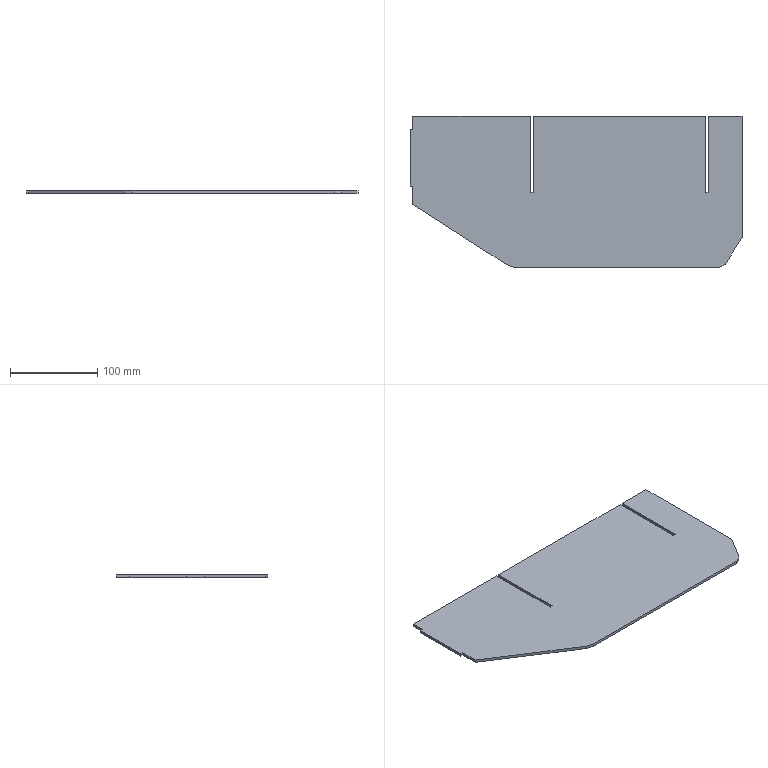Part | SolidWorks | features FlatPattern 1, SMBaseFlange 1, SheetMetal 1 | 1 solid | 22 faces | box 379.5 x 173.7 x 3.2 mm | volume 193629 mm3 | plane 22
STEP:
#1=CARTESIAN_POINT('',(-57.013,-111.363,0.));
#2=VERTEX_POINT('',#1);
#3=CARTESIAN_POINT('',(-47.809,-114.07,0.));
#4=VERTEX_POINT('',#3);
#5=CARTESIAN_POINT('',(-57.013,-111.363,0.));
#6=DIRECTION('',(0.9594,-0.2821,0.));
#7=VECTOR('',#6,1000.);
#8=LINE('',#5,#7);
#9=EDGE_CURVE('',#2,#4,#8,.T.);
#10=ORIENTED_EDGE('',*,*,#9,.T.);
#11=CARTESIAN_POINT('',(-47.809,-114.07,3.2));
#12=VERTEX_POINT('',#11);
#13=CARTESIAN_POINT('',(-47.809,-114.07,3.2));
#14=DIRECTION('',(0.,0.,-1.));
#15=VECTOR('',#14,1000.);
#16=LINE('',#13,#15);
#17=EDGE_CURVE('',#12,#4,#16,.T.);
#18=ORIENTED_EDGE('',*,*,#17,.F.);
#19=CARTESIAN_POINT('',(-57.013,-111.363,3.2));
#20=VERTEX_POINT('',#19);
#21=CARTESIAN_POINT('',(-57.013,-111.363,3.2));
#22=DIRECTION('',(0.9594,-0.2821,0.));
#23=VECTOR('',#22,1000.);
#24=LINE('',#21,#23);
#25=EDGE_CURVE('',#20,#12,#24,.T.);
#26=ORIENTED_EDGE('',*,*,#25,.F.);
#27=CARTESIAN_POINT('',(-57.013,-111.363,3.2));
#28=DIRECTION('',(0.,0.,-1.));
#29=VECTOR('',#28,1000.);
#30=LINE('',#27,#29);
#31=EDGE_CURVE('',#20,#2,#30,.T.);
#32=ORIENTED_EDGE('',*,*,#31,.T.);
#33=EDGE_LOOP('',(#10,#18,#26,#32));
#34=FACE_OUTER_BOUND('',#33,.T.);
#35=CARTESIAN_POINT('',(-57.013,-111.363,3.2));
#36=DIRECTION('',(0.2821,0.9594,0.));
#37=DIRECTION('',(-0.9594,0.2821,0.));
#38=AXIS2_PLACEMENT_3D('',#35,#36,#37);
#39=PLANE('',#38);
#40=ADVANCED_FACE('',(#34),#39,.F.);
#41=CARTESIAN_POINT('',(183.691,-114.07,0.));
#42=VERTEX_POINT('',#41);
#43=CARTESIAN_POINT('',(-47.809,-114.07,0.));
#44=DIRECTION('',(1.,0.,0.));
#45=VECTOR('',#44,1000.);
#46=LINE('',#43,#45);
#47=EDGE_CURVE('',#4,#42,#46,.T.);
#48=ORIENTED_EDGE('',*,*,#47,.T.);
#49=CARTESIAN_POINT('',(183.691,-114.07,3.2));
#50=VERTEX_POINT('',#49);
#51=CARTESIAN_POINT('',(183.691,-114.07,3.2));
#52=DIRECTION('',(0.,0.,-1.));
#53=VECTOR('',#52,1000.);
#54=LINE('',#51,#53);
#55=EDGE_CURVE('',#50,#42,#54,.T.);
#56=ORIENTED_EDGE('',*,*,#55,.F.);
#57=CARTESIAN_POINT('',(-47.809,-114.07,3.2));
#58=DIRECTION('',(1.,0.,0.));
#59=VECTOR('',#58,1000.);
#60=LINE('',#57,#59);
#61=EDGE_CURVE('',#12,#50,#60,.T.);
#62=ORIENTED_EDGE('',*,*,#61,.F.);
#63=ORIENTED_EDGE('',*,*,#17,.T.);
#64=EDGE_LOOP('',(#48,#56,#62,#63));
#65=FACE_OUTER_BOUND('',#64,.T.);
#66=CARTESIAN_POINT('',(-47.809,-114.07,3.2));
#67=DIRECTION('',(0.,1.,0.));
#68=DIRECTION('',(-1.,0.,0.));
#69=AXIS2_PLACEMENT_3D('',#66,#67,#68);
#70=PLANE('',#69);
#71=ADVANCED_FACE('',(#65),#70,.F.);
#72=CARTESIAN_POINT('',(191.335,-109.826,0.));
#73=VERTEX_POINT('',#72);
#74=CARTESIAN_POINT('',(183.691,-114.07,0.));
#75=DIRECTION('',(0.8743,0.4854,0.));
#76=VECTOR('',#75,1000.);
#77=LINE('',#74,#76);
#78=EDGE_CURVE('',#42,#73,#77,.T.);
#79=ORIENTED_EDGE('',*,*,#78,.T.);
#80=CARTESIAN_POINT('',(191.335,-109.826,3.2));
#81=VERTEX_POINT('',#80);
#82=CARTESIAN_POINT('',(191.335,-109.826,3.2));
#83=DIRECTION('',(0.,0.,-1.));
#84=VECTOR('',#83,1000.);
#85=LINE('',#82,#84);
#86=EDGE_CURVE('',#81,#73,#85,.T.);
#87=ORIENTED_EDGE('',*,*,#86,.F.);
#88=CARTESIAN_POINT('',(183.691,-114.07,3.2));
#89=DIRECTION('',(0.8743,0.4854,0.));
#90=VECTOR('',#89,1000.);
#91=LINE('',#88,#90);
#92=EDGE_CURVE('',#50,#81,#91,.T.);
#93=ORIENTED_EDGE('',*,*,#92,.F.);
#94=ORIENTED_EDGE('',*,*,#55,.T.);
#95=EDGE_LOOP('',(#79,#87,#93,#94));
#96=FACE_OUTER_BOUND('',#95,.T.);
#97=CARTESIAN_POINT('',(183.691,-114.07,3.2));
#98=DIRECTION('',(-0.4854,0.8743,0.));
#99=DIRECTION('',(-0.8743,-0.4854,0.));
#100=AXIS2_PLACEMENT_3D('',#97,#98,#99);
#101=PLANE('',#100);
#102=ADVANCED_FACE('',(#96),#101,.F.);
#103=CARTESIAN_POINT('',(210.391,-79.24,0.));
#104=VERTEX_POINT('',#103);
#105=CARTESIAN_POINT('',(191.335,-109.826,0.));
#106=DIRECTION('',(0.5288,0.8487,0.));
#107=VECTOR('',#106,1000.);
#108=LINE('',#105,#107);
#109=EDGE_CURVE('',#73,#104,#108,.T.);
#110=ORIENTED_EDGE('',*,*,#109,.T.);
#111=CARTESIAN_POINT('',(210.391,-79.24,3.2));
#112=VERTEX_POINT('',#111);
#113=CARTESIAN_POINT('',(210.391,-79.24,3.2));
#114=DIRECTION('',(0.,0.,-1.));
#115=VECTOR('',#114,1000.);
#116=LINE('',#113,#115);
#117=EDGE_CURVE('',#112,#104,#116,.T.);
#118=ORIENTED_EDGE('',*,*,#117,.F.);
#119=CARTESIAN_POINT('',(191.335,-109.826,3.2));
#120=DIRECTION('',(0.5288,0.8487,0.));
#121=VECTOR('',#120,1000.);
#122=LINE('',#119,#121);
#123=EDGE_CURVE('',#81,#112,#122,.T.);
#124=ORIENTED_EDGE('',*,*,#123,.F.);
#125=ORIENTED_EDGE('',*,*,#86,.T.);
#126=EDGE_LOOP('',(#110,#118,#124,#125));
#127=FACE_OUTER_BOUND('',#126,.T.);
#128=CARTESIAN_POINT('',(191.335,-109.826,3.2));
#129=DIRECTION('',(-0.8487,0.5288,0.));
#130=DIRECTION('',(-0.5288,-0.8487,0.));
#131=AXIS2_PLACEMENT_3D('',#128,#129,#130);
#132=PLANE('',#131);
#133=ADVANCED_FACE('',(#127),#132,.F.);
#134=CARTESIAN_POINT('',(210.391,59.63,0.));
#135=VERTEX_POINT('',#134);
#136=CARTESIAN_POINT('',(210.391,-79.24,0.));
#137=DIRECTION('',(0.,1.,0.));
#138=VECTOR('',#137,1000.);
#139=LINE('',#136,#138);
#140=EDGE_CURVE('',#104,#135,#139,.T.);
#141=ORIENTED_EDGE('',*,*,#140,.T.);
#142=CARTESIAN_POINT('',(210.391,59.63,3.2));
#143=VERTEX_POINT('',#142);
#144=CARTESIAN_POINT('',(210.391,59.63,3.2));
#145=DIRECTION('',(0.,0.,-1.));
#146=VECTOR('',#145,1000.);
#147=LINE('',#144,#146);
#148=EDGE_CURVE('',#143,#135,#147,.T.);
#149=ORIENTED_EDGE('',*,*,#148,.F.);
#150=CARTESIAN_POINT('',(210.391,-79.24,3.2));
#151=DIRECTION('',(0.,1.,0.));
#152=VECTOR('',#151,1000.);
#153=LINE('',#150,#152);
#154=EDGE_CURVE('',#112,#143,#153,.T.);
#155=ORIENTED_EDGE('',*,*,#154,.F.);
#156=ORIENTED_EDGE('',*,*,#117,.T.);
#157=EDGE_LOOP('',(#141,#149,#155,#156));
#158=FACE_OUTER_BOUND('',#157,.T.);
#159=CARTESIAN_POINT('',(210.391,-79.24,3.2));
#160=DIRECTION('',(-1.,0.,0.));
#161=DIRECTION('',(0.,0.,1.));
#162=AXIS2_PLACEMENT_3D('',#159,#160,#161);
#163=PLANE('',#162);
#164=ADVANCED_FACE('',(#158),#163,.F.);
#165=CARTESIAN_POINT('',(171.891,59.63,0.));
#166=VERTEX_POINT('',#165);
#167=CARTESIAN_POINT('',(171.891,59.63,0.));
#168=DIRECTION('',(-1.,0.,0.));
#169=VECTOR('',#168,1000.);
#170=LINE('',#167,#169);
#171=EDGE_CURVE('',#135,#166,#170,.T.);
#172=ORIENTED_EDGE('',*,*,#171,.T.);
#173=CARTESIAN_POINT('',(171.891,59.63,3.2));
#174=VERTEX_POINT('',#173);
#175=CARTESIAN_POINT('',(171.891,59.63,3.2));
#176=DIRECTION('',(0.,0.,-1.));
#177=VECTOR('',#176,1000.);
#178=LINE('',#175,#177);
#179=EDGE_CURVE('',#174,#166,#178,.T.);
#180=ORIENTED_EDGE('',*,*,#179,.F.);
#181=CARTESIAN_POINT('',(171.891,59.63,3.2));
#182=DIRECTION('',(-1.,0.,0.));
#183=VECTOR('',#182,1000.);
#184=LINE('',#181,#183);
#185=EDGE_CURVE('',#143,#174,#184,.T.);
#186=ORIENTED_EDGE('',*,*,#185,.F.);
#187=ORIENTED_EDGE('',*,*,#148,.T.);
#188=EDGE_LOOP('',(#172,#180,#186,#187));
#189=FACE_OUTER_BOUND('',#188,.T.);
#190=CARTESIAN_POINT('',(171.891,59.63,3.2));
#191=DIRECTION('',(0.,-1.,0.));
#192=DIRECTION('',(0.,0.,-1.));
#193=AXIS2_PLACEMENT_3D('',#190,#191,#192);
#194=PLANE('',#193);
#195=ADVANCED_FACE('',(#189),#194,.F.);
#196=CARTESIAN_POINT('',(171.891,-27.37,0.));
#197=VERTEX_POINT('',#196);
#198=CARTESIAN_POINT('',(171.891,-27.37,0.));
#199=DIRECTION('',(0.,-1.,0.));
#200=VECTOR('',#199,1000.);
#201=LINE('',#198,#200);
#202=EDGE_CURVE('',#166,#197,#201,.T.);
#203=ORIENTED_EDGE('',*,*,#202,.T.);
#204=CARTESIAN_POINT('',(171.891,-27.37,3.2));
#205=VERTEX_POINT('',#204);
#206=CARTESIAN_POINT('',(171.891,-27.37,3.2));
#207=DIRECTION('',(0.,0.,-1.));
#208=VECTOR('',#207,1000.);
#209=LINE('',#206,#208);
#210=EDGE_CURVE('',#205,#197,#209,.T.);
#211=ORIENTED_EDGE('',*,*,#210,.F.);
#212=CARTESIAN_POINT('',(171.891,-27.37,3.2));
#213=DIRECTION('',(0.,-1.,0.));
#214=VECTOR('',#213,1000.);
#215=LINE('',#212,#214);
#216=EDGE_CURVE('',#174,#205,#215,.T.);
#217=ORIENTED_EDGE('',*,*,#216,.F.);
#218=ORIENTED_EDGE('',*,*,#179,.T.);
#219=EDGE_LOOP('',(#203,#211,#217,#218));
#220=FACE_OUTER_BOUND('',#219,.T.);
#221=CARTESIAN_POINT('',(171.891,-27.37,3.2));
#222=DIRECTION('',(1.,0.,0.));
#223=DIRECTION('',(0.,1.,0.));
#224=AXIS2_PLACEMENT_3D('',#221,#222,#223);
#225=PLANE('',#224);
#226=ADVANCED_FACE('',(#220),#225,.F.);
#227=CARTESIAN_POINT('',(168.691,-27.37,0.));
#228=VERTEX_POINT('',#227);
#229=CARTESIAN_POINT('',(168.691,-27.37,0.));
#230=DIRECTION('',(-1.,0.,0.));
#231=VECTOR('',#230,1000.);
#232=LINE('',#229,#231);
#233=EDGE_CURVE('',#197,#228,#232,.T.);
#234=ORIENTED_EDGE('',*,*,#233,.T.);
#235=CARTESIAN_POINT('',(168.691,-27.37,3.2));
#236=VERTEX_POINT('',#235);
#237=CARTESIAN_POINT('',(168.691,-27.37,3.2));
#238=DIRECTION('',(0.,0.,-1.));
#239=VECTOR('',#238,1000.);
#240=LINE('',#237,#239);
#241=EDGE_CURVE('',#236,#228,#240,.T.);
#242=ORIENTED_EDGE('',*,*,#241,.F.);
#243=CARTESIAN_POINT('',(168.691,-27.37,3.2));
#244=DIRECTION('',(-1.,0.,0.));
#245=VECTOR('',#244,1000.);
#246=LINE('',#243,#245);
#247=EDGE_CURVE('',#205,#236,#246,.T.);
#248=ORIENTED_EDGE('',*,*,#247,.F.);
#249=ORIENTED_EDGE('',*,*,#210,.T.);
#250=EDGE_LOOP('',(#234,#242,#248,#249));
#251=FACE_OUTER_BOUND('',#250,.T.);
#252=CARTESIAN_POINT('',(168.691,-27.37,3.2));
#253=DIRECTION('',(0.,-1.,0.));
#254=DIRECTION('',(0.,0.,-1.));
#255=AXIS2_PLACEMENT_3D('',#252,#253,#254);
#256=PLANE('',#255);
#257=ADVANCED_FACE('',(#251),#256,.F.);
#258=CARTESIAN_POINT('',(168.691,59.63,0.));
#259=VERTEX_POINT('',#258);
#260=CARTESIAN_POINT('',(168.691,59.63,0.));
#261=DIRECTION('',(0.,1.,0.));
#262=VECTOR('',#261,1000.);
#263=LINE('',#260,#262);
#264=EDGE_CURVE('',#228,#259,#263,.T.);
#265=ORIENTED_EDGE('',*,*,#264,.T.);
#266=CARTESIAN_POINT('',(168.691,59.63,3.2));
#267=VERTEX_POINT('',#266);
#268=CARTESIAN_POINT('',(168.691,59.63,3.2));
#269=DIRECTION('',(0.,0.,-1.));
#270=VECTOR('',#269,1000.);
#271=LINE('',#268,#270);
#272=EDGE_CURVE('',#267,#259,#271,.T.);
#273=ORIENTED_EDGE('',*,*,#272,.F.);
#274=CARTESIAN_POINT('',(168.691,59.63,3.2));
#275=DIRECTION('',(0.,1.,0.));
#276=VECTOR('',#275,1000.);
#277=LINE('',#274,#276);
#278=EDGE_CURVE('',#236,#267,#277,.T.);
#279=ORIENTED_EDGE('',*,*,#278,.F.);
#280=ORIENTED_EDGE('',*,*,#241,.T.);
#281=EDGE_LOOP('',(#265,#273,#279,#280));
#282=FACE_OUTER_BOUND('',#281,.T.);
#283=CARTESIAN_POINT('',(168.691,59.63,3.2));
#284=DIRECTION('',(-1.,0.,0.));
#285=DIRECTION('',(0.,0.,1.));
#286=AXIS2_PLACEMENT_3D('',#283,#284,#285);
#287=PLANE('',#286);
#288=ADVANCED_FACE('',(#282),#287,.F.);
#289=CARTESIAN_POINT('',(-28.109,59.63,0.));
#290=VERTEX_POINT('',#289);
#291=CARTESIAN_POINT('',(-28.109,59.63,0.));
#292=DIRECTION('',(-1.,0.,0.));
#293=VECTOR('',#292,1000.);
#294=LINE('',#291,#293);
#295=EDGE_CURVE('',#259,#290,#294,.T.);
#296=ORIENTED_EDGE('',*,*,#295,.T.);
#297=CARTESIAN_POINT('',(-28.109,59.63,3.2));
#298=VERTEX_POINT('',#297);
#299=CARTESIAN_POINT('',(-28.109,59.63,3.2));
#300=DIRECTION('',(0.,0.,-1.));
#301=VECTOR('',#300,1000.);
#302=LINE('',#299,#301);
#303=EDGE_CURVE('',#298,#290,#302,.T.);
#304=ORIENTED_EDGE('',*,*,#303,.F.);
#305=CARTESIAN_POINT('',(-28.109,59.63,3.2));
#306=DIRECTION('',(-1.,0.,0.));
#307=VECTOR('',#306,1000.);
#308=LINE('',#305,#307);
#309=EDGE_CURVE('',#267,#298,#308,.T.);
#310=ORIENTED_EDGE('',*,*,#309,.F.);
#311=ORIENTED_EDGE('',*,*,#272,.T.);
#312=EDGE_LOOP('',(#296,#304,#310,#311));
#313=FACE_OUTER_BOUND('',#312,.T.);
#314=CARTESIAN_POINT('',(-28.109,59.63,3.2));
#315=DIRECTION('',(0.,-1.,0.));
#316=DIRECTION('',(0.,0.,-1.));
#317=AXIS2_PLACEMENT_3D('',#314,#315,#316);
#318=PLANE('',#317);
#319=ADVANCED_FACE('',(#313),#318,.F.);
#320=CARTESIAN_POINT('',(-28.109,-27.37,0.));
#321=VERTEX_POINT('',#320);
#322=CARTESIAN_POINT('',(-28.109,-27.37,0.));
#323=DIRECTION('',(0.,-1.,0.));
#324=VECTOR('',#323,1000.);
#325=LINE('',#322,#324);
#326=EDGE_CURVE('',#290,#321,#325,.T.);
#327=ORIENTED_EDGE('',*,*,#326,.T.);
#328=CARTESIAN_POINT('',(-28.109,-27.37,3.2));
#329=VERTEX_POINT('',#328);
#330=CARTESIAN_POINT('',(-28.109,-27.37,3.2));
#331=DIRECTION('',(0.,0.,-1.));
#332=VECTOR('',#331,1000.);
#333=LINE('',#330,#332);
#334=EDGE_CURVE('',#329,#321,#333,.T.);
#335=ORIENTED_EDGE('',*,*,#334,.F.);
#336=CARTESIAN_POINT('',(-28.109,-27.37,3.2));
#337=DIRECTION('',(0.,-1.,0.));
#338=VECTOR('',#337,1000.);
#339=LINE('',#336,#338);
#340=EDGE_CURVE('',#298,#329,#339,.T.);
#341=ORIENTED_EDGE('',*,*,#340,.F.);
#342=ORIENTED_EDGE('',*,*,#303,.T.);
#343=EDGE_LOOP('',(#327,#335,#341,#342));
#344=FACE_OUTER_BOUND('',#343,.T.);
#345=CARTESIAN_POINT('',(-28.109,-27.37,3.2));
#346=DIRECTION('',(1.,0.,0.));
#347=DIRECTION('',(0.,1.,0.));
#348=AXIS2_PLACEMENT_3D('',#345,#346,#347);
#349=PLANE('',#348);
#350=ADVANCED_FACE('',(#344),#349,.F.);
#351=CARTESIAN_POINT('',(-31.309,-27.37,0.));
#352=VERTEX_POINT('',#351);
#353=CARTESIAN_POINT('',(-31.309,-27.37,0.));
#354=DIRECTION('',(-1.,0.,0.));
#355=VECTOR('',#354,1000.);
#356=LINE('',#353,#355);
#357=EDGE_CURVE('',#321,#352,#356,.T.);
#358=ORIENTED_EDGE('',*,*,#357,.T.);
#359=CARTESIAN_POINT('',(-31.309,-27.37,3.2));
#360=VERTEX_POINT('',#359);
#361=CARTESIAN_POINT('',(-31.309,-27.37,3.2));
#362=DIRECTION('',(0.,0.,-1.));
#363=VECTOR('',#362,1000.);
#364=LINE('',#361,#363);
#365=EDGE_CURVE('',#360,#352,#364,.T.);
#366=ORIENTED_EDGE('',*,*,#365,.F.);
#367=CARTESIAN_POINT('',(-31.309,-27.37,3.2));
#368=DIRECTION('',(-1.,0.,0.));
#369=VECTOR('',#368,1000.);
#370=LINE('',#367,#369);
#371=EDGE_CURVE('',#329,#360,#370,.T.);
#372=ORIENTED_EDGE('',*,*,#371,.F.);
#373=ORIENTED_EDGE('',*,*,#334,.T.);
#374=EDGE_LOOP('',(#358,#366,#372,#373));
#375=FACE_OUTER_BOUND('',#374,.T.);
#376=CARTESIAN_POINT('',(-31.309,-27.37,3.2));
#377=DIRECTION('',(0.,-1.,0.));
#378=DIRECTION('',(0.,0.,-1.));
#379=AXIS2_PLACEMENT_3D('',#376,#377,#378);
#380=PLANE('',#379);
#381=ADVANCED_FACE('',(#375),#380,.F.);
#382=CARTESIAN_POINT('',(-31.309,59.63,0.));
#383=VERTEX_POINT('',#382);
#384=CARTESIAN_POINT('',(-31.309,59.63,0.));
#385=DIRECTION('',(0.,1.,0.));
#386=VECTOR('',#385,1000.);
#387=LINE('',#384,#386);
#388=EDGE_CURVE('',#352,#383,#387,.T.);
#389=ORIENTED_EDGE('',*,*,#388,.T.);
#390=CARTESIAN_POINT('',(-31.309,59.63,3.2));
#391=VERTEX_POINT('',#390);
#392=CARTESIAN_POINT('',(-31.309,59.63,3.2));
#393=DIRECTION('',(0.,0.,-1.));
#394=VECTOR('',#393,1000.);
#395=LINE('',#392,#394);
#396=EDGE_CURVE('',#391,#383,#395,.T.);
#397=ORIENTED_EDGE('',*,*,#396,.F.);
#398=CARTESIAN_POINT('',(-31.309,59.63,3.2));
#399=DIRECTION('',(0.,1.,0.));
#400=VECTOR('',#399,1000.);
#401=LINE('',#398,#400);
#402=EDGE_CURVE('',#360,#391,#401,.T.);
#403=ORIENTED_EDGE('',*,*,#402,.F.);
#404=ORIENTED_EDGE('',*,*,#365,.T.);
#405=EDGE_LOOP('',(#389,#397,#403,#404));
#406=FACE_OUTER_BOUND('',#405,.T.);
#407=CARTESIAN_POINT('',(-31.309,59.63,3.2));
#408=DIRECTION('',(-1.,0.,0.));
#409=DIRECTION('',(0.,-1.,0.));
#410=AXIS2_PLACEMENT_3D('',#407,#408,#409);
#411=PLANE('',#410);
#412=ADVANCED_FACE('',(#406),#411,.F.);
#413=CARTESIAN_POINT('',(-166.109,59.63,0.));
#414=VERTEX_POINT('',#413);
#415=CARTESIAN_POINT('',(-166.109,59.63,0.));
#416=DIRECTION('',(-1.,0.,0.));
#417=VECTOR('',#416,1000.);
#418=LINE('',#415,#417);
#419=EDGE_CURVE('',#383,#414,#418,.T.);
#420=ORIENTED_EDGE('',*,*,#419,.T.);
#421=CARTESIAN_POINT('',(-166.109,59.63,3.2));
#422=VERTEX_POINT('',#421);
#423=CARTESIAN_POINT('',(-166.109,59.63,3.2));
#424=DIRECTION('',(0.,0.,-1.));
#425=VECTOR('',#424,1000.);
#426=LINE('',#423,#425);
#427=EDGE_CURVE('',#422,#414,#426,.T.);
#428=ORIENTED_EDGE('',*,*,#427,.F.);
#429=CARTESIAN_POINT('',(-166.109,59.63,3.2));
#430=DIRECTION('',(-1.,0.,0.));
#431=VECTOR('',#430,1000.);
#432=LINE('',#429,#431);
#433=EDGE_CURVE('',#391,#422,#432,.T.);
#434=ORIENTED_EDGE('',*,*,#433,.F.);
#435=ORIENTED_EDGE('',*,*,#396,.T.);
#436=EDGE_LOOP('',(#420,#428,#434,#435));
#437=FACE_OUTER_BOUND('',#436,.T.);
#438=CARTESIAN_POINT('',(-166.109,59.63,3.2));
#439=DIRECTION('',(0.,-1.,0.));
#440=DIRECTION('',(0.,0.,-1.));
#441=AXIS2_PLACEMENT_3D('',#438,#439,#440);
#442=PLANE('',#441);
#443=ADVANCED_FACE('',(#437),#442,.F.);
#444=CARTESIAN_POINT('',(-166.109,44.63,0.));
#445=VERTEX_POINT('',#444);
#446=CARTESIAN_POINT('',(-166.109,59.63,0.));
#447=DIRECTION('',(0.,-1.,0.));
#448=VECTOR('',#447,1000.);
#449=LINE('',#446,#448);
#450=EDGE_CURVE('',#414,#445,#449,.T.);
#451=ORIENTED_EDGE('',*,*,#450,.T.);
#452=CARTESIAN_POINT('',(-166.109,44.63,3.2));
#453=VERTEX_POINT('',#452);
#454=CARTESIAN_POINT('',(-166.109,44.63,3.2));
#455=DIRECTION('',(0.,0.,-1.));
#456=VECTOR('',#455,1000.);
#457=LINE('',#454,#456);
#458=EDGE_CURVE('',#453,#445,#457,.T.);
#459=ORIENTED_EDGE('',*,*,#458,.F.);
#460=CARTESIAN_POINT('',(-166.109,59.63,3.2));
#461=DIRECTION('',(0.,-1.,0.));
#462=VECTOR('',#461,1000.);
#463=LINE('',#460,#462);
#464=EDGE_CURVE('',#422,#453,#463,.T.);
#465=ORIENTED_EDGE('',*,*,#464,.F.);
#466=ORIENTED_EDGE('',*,*,#427,.T.);
#467=EDGE_LOOP('',(#451,#459,#465,#466));
#468=FACE_OUTER_BOUND('',#467,.T.);
#469=CARTESIAN_POINT('',(-166.109,59.63,3.2));
#470=DIRECTION('',(1.,0.,0.));
#471=DIRECTION('',(0.,1.,0.));
#472=AXIS2_PLACEMENT_3D('',#469,#470,#471);
#473=PLANE('',#472);
#474=ADVANCED_FACE('',(#468),#473,.F.);
#475=CARTESIAN_POINT('',(-169.109,44.63,0.));
#476=VERTEX_POINT('',#475);
#477=CARTESIAN_POINT('',(-169.109,44.63,0.));
#478=DIRECTION('',(-1.,0.,0.));
#479=VECTOR('',#478,1000.);
#480=LINE('',#477,#479);
#481=EDGE_CURVE('',#445,#476,#480,.T.);
#482=ORIENTED_EDGE('',*,*,#481,.T.);
#483=CARTESIAN_POINT('',(-169.109,44.63,3.2));
#484=VERTEX_POINT('',#483);
#485=CARTESIAN_POINT('',(-169.109,44.63,3.2));
#486=DIRECTION('',(0.,0.,-1.));
#487=VECTOR('',#486,1000.);
#488=LINE('',#485,#487);
#489=EDGE_CURVE('',#484,#476,#488,.T.);
#490=ORIENTED_EDGE('',*,*,#489,.F.);
#491=CARTESIAN_POINT('',(-169.109,44.63,3.2));
#492=DIRECTION('',(-1.,0.,0.));
#493=VECTOR('',#492,1000.);
#494=LINE('',#491,#493);
#495=EDGE_CURVE('',#453,#484,#494,.T.);
#496=ORIENTED_EDGE('',*,*,#495,.F.);
#497=ORIENTED_EDGE('',*,*,#458,.T.);
#498=EDGE_LOOP('',(#482,#490,#496,#497));
#499=FACE_OUTER_BOUND('',#498,.T.);
#500=CARTESIAN_POINT('',(-169.109,44.63,3.2));
#501=DIRECTION('',(0.,-1.,0.));
#502=DIRECTION('',(0.,0.,-1.));
#503=AXIS2_PLACEMENT_3D('',#500,#501,#502);
#504=PLANE('',#503);
#505=ADVANCED_FACE('',(#499),#504,.F.);
#506=CARTESIAN_POINT('',(-169.109,-20.37,0.));
#507=VERTEX_POINT('',#506);
#508=CARTESIAN_POINT('',(-169.109,-20.37,0.));
#509=DIRECTION('',(0.,-1.,0.));
#510=VECTOR('',#509,1000.);
#511=LINE('',#508,#510);
#512=EDGE_CURVE('',#476,#507,#511,.T.);
#513=ORIENTED_EDGE('',*,*,#512,.T.);
#514=CARTESIAN_POINT('',(-169.109,-20.37,3.2));
#515=VERTEX_POINT('',#514);
#516=CARTESIAN_POINT('',(-169.109,-20.37,3.2));
#517=DIRECTION('',(0.,0.,-1.));
#518=VECTOR('',#517,1000.);
#519=LINE('',#516,#518);
#520=EDGE_CURVE('',#515,#507,#519,.T.);
#521=ORIENTED_EDGE('',*,*,#520,.F.);
#522=CARTESIAN_POINT('',(-169.109,-20.37,3.2));
#523=DIRECTION('',(0.,-1.,0.));
#524=VECTOR('',#523,1000.);
#525=LINE('',#522,#524);
#526=EDGE_CURVE('',#484,#515,#525,.T.);
#527=ORIENTED_EDGE('',*,*,#526,.F.);
#528=ORIENTED_EDGE('',*,*,#489,.T.);
#529=EDGE_LOOP('',(#513,#521,#527,#528));
#530=FACE_OUTER_BOUND('',#529,.T.);
#531=CARTESIAN_POINT('',(-169.109,-20.37,3.2));
#532=DIRECTION('',(1.,0.,0.));
#533=DIRECTION('',(0.,0.,-1.));
#534=AXIS2_PLACEMENT_3D('',#531,#532,#533);
#535=PLANE('',#534);
#536=ADVANCED_FACE('',(#530),#535,.F.);
#537=CARTESIAN_POINT('',(-166.109,-20.37,0.));
#538=VERTEX_POINT('',#537);
#539=CARTESIAN_POINT('',(-166.109,-20.37,0.));
#540=DIRECTION('',(1.,0.,0.));
#541=VECTOR('',#540,1000.);
#542=LINE('',#539,#541);
#543=EDGE_CURVE('',#507,#538,#542,.T.);
#544=ORIENTED_EDGE('',*,*,#543,.T.);
#545=CARTESIAN_POINT('',(-166.109,-20.37,3.2));
#546=VERTEX_POINT('',#545);
#547=CARTESIAN_POINT('',(-166.109,-20.37,3.2));
#548=DIRECTION('',(0.,0.,-1.));
#549=VECTOR('',#548,1000.);
#550=LINE('',#547,#549);
#551=EDGE_CURVE('',#546,#538,#550,.T.);
#552=ORIENTED_EDGE('',*,*,#551,.F.);
#553=CARTESIAN_POINT('',(-166.109,-20.37,3.2));
#554=DIRECTION('',(1.,0.,0.));
#555=VECTOR('',#554,1000.);
#556=LINE('',#553,#555);
#557=EDGE_CURVE('',#515,#546,#556,.T.);
#558=ORIENTED_EDGE('',*,*,#557,.F.);
#559=ORIENTED_EDGE('',*,*,#520,.T.);
#560=EDGE_LOOP('',(#544,#552,#558,#559));
#561=FACE_OUTER_BOUND('',#560,.T.);
#562=CARTESIAN_POINT('',(-166.109,-20.37,3.2));
#563=DIRECTION('',(0.,1.,0.));
#564=DIRECTION('',(0.,0.,1.));
#565=AXIS2_PLACEMENT_3D('',#562,#563,#564);
#566=PLANE('',#565);
#567=ADVANCED_FACE('',(#561),#566,.F.);
#568=CARTESIAN_POINT('',(-166.109,-41.13,0.));
#569=VERTEX_POINT('',#568);
#570=CARTESIAN_POINT('',(-166.109,-20.37,0.));
#571=DIRECTION('',(0.,-1.,0.));
#572=VECTOR('',#571,1000.);
#573=LINE('',#570,#572);
#574=EDGE_CURVE('',#538,#569,#573,.T.);
#575=ORIENTED_EDGE('',*,*,#574,.T.);
#576=CARTESIAN_POINT('',(-166.109,-41.13,3.2));
#577=VERTEX_POINT('',#576);
#578=CARTESIAN_POINT('',(-166.109,-41.13,3.2));
#579=DIRECTION('',(0.,0.,-1.));
#580=VECTOR('',#579,1000.);
#581=LINE('',#578,#580);
#582=EDGE_CURVE('',#577,#569,#581,.T.);
#583=ORIENTED_EDGE('',*,*,#582,.F.);
#584=CARTESIAN_POINT('',(-166.109,-20.37,3.2));
#585=DIRECTION('',(0.,-1.,0.));
#586=VECTOR('',#585,1000.);
#587=LINE('',#584,#586);
#588=EDGE_CURVE('',#546,#577,#587,.T.);
#589=ORIENTED_EDGE('',*,*,#588,.F.);
#590=ORIENTED_EDGE('',*,*,#551,.T.);
#591=EDGE_LOOP('',(#575,#583,#589,#590));
#592=FACE_OUTER_BOUND('',#591,.T.);
#593=CARTESIAN_POINT('',(-166.109,-20.37,3.2));
#594=DIRECTION('',(1.,0.,0.));
#595=DIRECTION('',(0.,1.,0.));
#596=AXIS2_PLACEMENT_3D('',#593,#594,#595);
#597=PLANE('',#596);
#598=ADVANCED_FACE('',(#592),#597,.F.);
#599=CARTESIAN_POINT('',(-166.109,-41.13,0.));
#600=DIRECTION('',(0.8408,-0.5413,0.));
#601=VECTOR('',#600,1000.);
#602=LINE('',#599,#601);
#603=EDGE_CURVE('',#569,#2,#602,.T.);
#604=ORIENTED_EDGE('',*,*,#603,.T.);
#605=ORIENTED_EDGE('',*,*,#31,.F.);
#606=CARTESIAN_POINT('',(-166.109,-41.13,3.2));
#607=DIRECTION('',(0.8408,-0.5413,0.));
#608=VECTOR('',#607,1000.);
#609=LINE('',#606,#608);
#610=EDGE_CURVE('',#577,#20,#609,.T.);
#611=ORIENTED_EDGE('',*,*,#610,.F.);
#612=ORIENTED_EDGE('',*,*,#582,.T.);
#613=EDGE_LOOP('',(#604,#605,#611,#612));
#614=FACE_OUTER_BOUND('',#613,.T.);
#615=CARTESIAN_POINT('',(-166.109,-41.13,3.2));
#616=DIRECTION('',(0.5413,0.8408,0.));
#617=DIRECTION('',(-0.8408,0.5413,0.));
#618=AXIS2_PLACEMENT_3D('',#615,#616,#617);
#619=PLANE('',#618);
#620=ADVANCED_FACE('',(#614),#619,.F.);
#621=ORIENTED_EDGE('',*,*,#25,.T.);
#622=ORIENTED_EDGE('',*,*,#61,.T.);
#623=ORIENTED_EDGE('',*,*,#92,.T.);
#624=ORIENTED_EDGE('',*,*,#123,.T.);
#625=ORIENTED_EDGE('',*,*,#154,.T.);
#626=ORIENTED_EDGE('',*,*,#185,.T.);
#627=ORIENTED_EDGE('',*,*,#216,.T.);
#628=ORIENTED_EDGE('',*,*,#247,.T.);
#629=ORIENTED_EDGE('',*,*,#278,.T.);
#630=ORIENTED_EDGE('',*,*,#309,.T.);
#631=ORIENTED_EDGE('',*,*,#340,.T.);
#632=ORIENTED_EDGE('',*,*,#371,.T.);
#633=ORIENTED_EDGE('',*,*,#402,.T.);
#634=ORIENTED_EDGE('',*,*,#433,.T.);
#635=ORIENTED_EDGE('',*,*,#464,.T.);
#636=ORIENTED_EDGE('',*,*,#495,.T.);
#637=ORIENTED_EDGE('',*,*,#526,.T.);
#638=ORIENTED_EDGE('',*,*,#557,.T.);
#639=ORIENTED_EDGE('',*,*,#588,.T.);
#640=ORIENTED_EDGE('',*,*,#610,.T.);
#641=EDGE_LOOP('',(#621,#622,#623,#624,#625,#626,#627,#628,#629,#630,#631,#632,#633,#634,#635,#636,#637,#638,#639,#640));
#642=FACE_OUTER_BOUND('',#641,.T.);
#643=CARTESIAN_POINT('',(0.,0.,3.2));
#644=DIRECTION('',(0.,0.,1.));
#645=DIRECTION('',(1.,0.,0.));
#646=AXIS2_PLACEMENT_3D('',#643,#644,#645);
#647=PLANE('',#646);
#648=ADVANCED_FACE('',(#642),#647,.T.);
#649=ORIENTED_EDGE('',*,*,#9,.F.);
#650=ORIENTED_EDGE('',*,*,#603,.F.);
#651=ORIENTED_EDGE('',*,*,#574,.F.);
#652=ORIENTED_EDGE('',*,*,#543,.F.);
#653=ORIENTED_EDGE('',*,*,#512,.F.);
#654=ORIENTED_EDGE('',*,*,#481,.F.);
#655=ORIENTED_EDGE('',*,*,#450,.F.);
#656=ORIENTED_EDGE('',*,*,#419,.F.);
#657=ORIENTED_EDGE('',*,*,#388,.F.);
#658=ORIENTED_EDGE('',*,*,#357,.F.);
#659=ORIENTED_EDGE('',*,*,#326,.F.);
#660=ORIENTED_EDGE('',*,*,#295,.F.);
#661=ORIENTED_EDGE('',*,*,#264,.F.);
#662=ORIENTED_EDGE('',*,*,#233,.F.);
#663=ORIENTED_EDGE('',*,*,#202,.F.);
#664=ORIENTED_EDGE('',*,*,#171,.F.);
#665=ORIENTED_EDGE('',*,*,#140,.F.);
#666=ORIENTED_EDGE('',*,*,#109,.F.);
#667=ORIENTED_EDGE('',*,*,#78,.F.);
#668=ORIENTED_EDGE('',*,*,#47,.F.);
#669=EDGE_LOOP('',(#649,#650,#651,#652,#653,#654,#655,#656,#657,#658,#659,#660,#661,#662,#663,#664,#665,#666,#667,#668));
#670=FACE_OUTER_BOUND('',#669,.T.);
#671=CARTESIAN_POINT('',(0.,0.,0.));
#672=DIRECTION('',(0.,0.,1.));
#673=DIRECTION('',(1.,0.,0.));
#674=AXIS2_PLACEMENT_3D('',#671,#672,#673);
#675=PLANE('',#674);
#676=ADVANCED_FACE('',(#670),#675,.F.);
#677=CLOSED_SHELL('',(#40,#71,#102,#133,#164,#195,#226,#257,#288,#319,#350,#381,#412,#443,#474,#505,#536,#567,#598,#620,#648,#676));
#678=MANIFOLD_SOLID_BREP('',#677);
#679=CARTESIAN_POINT('',(0.,0.,0.));
#680=DIRECTION('',(0.,0.,1.));
#681=DIRECTION('',(1.,0.,0.));
#682=AXIS2_PLACEMENT_3D('',#679,#680,#681);
#683=(LENGTH_UNIT()NAMED_UNIT(*)SI_UNIT(.MILLI.,.METRE.));
#684=UNCERTAINTY_MEASURE_WITH_UNIT(LENGTH_MEASURE(0.00001),#683,'','');
#685=(NAMED_UNIT(*)PLANE_ANGLE_UNIT()SI_UNIT($,.RADIAN.));
#686=(NAMED_UNIT(*)SI_UNIT($,.STERADIAN.)SOLID_ANGLE_UNIT());
#687=(GEOMETRIC_REPRESENTATION_CONTEXT(3)GLOBAL_UNCERTAINTY_ASSIGNED_CONTEXT((#684))GLOBAL_UNIT_ASSIGNED_CONTEXT((#683,#685,#686))REPRESENTATION_CONTEXT('',''));
#688=ADVANCED_BREP_SHAPE_REPRESENTATION('',(#678,#682),#687);